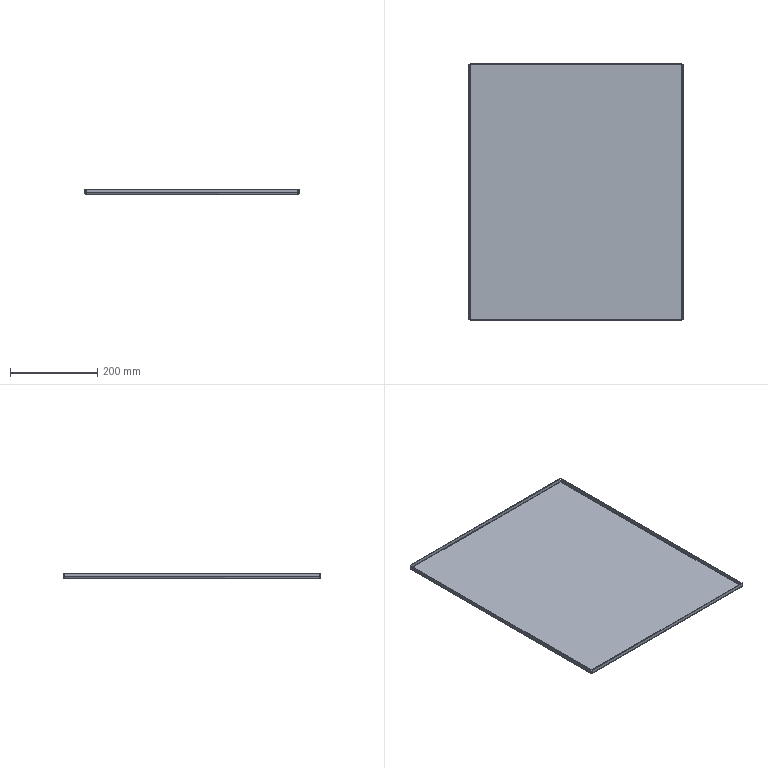Part | SolidWorks | features EdgeFlange 1, FlatPattern 1, SMBaseFlange 1, SheetMetal 1 | 1 solid | 38 faces | box 490 x 590 x 10 mm | volume 609167 mm3 | plane 22 | spline 8 | cylinder 8 | commonest cylinder face diameters 1.473 x4 5.473 x4
STEP:
#1=CARTESIAN_POINT('',(242.263,292.263,-2.));
#2=VERTEX_POINT('',#1);
#3=CARTESIAN_POINT('',(242.263,-292.263,-2.));
#4=VERTEX_POINT('',#3);
#5=CARTESIAN_POINT('',(242.263,292.293,-2.));
#6=DIRECTION('',(0.,-1.,0.));
#7=VECTOR('',#6,1000.);
#8=LINE('',#5,#7);
#9=EDGE_CURVE('',#2,#4,#8,.T.);
#10=ORIENTED_EDGE('',*,*,#9,.T.);
#11=CARTESIAN_POINT('',(-242.263,-292.263,-2.));
#12=VERTEX_POINT('',#11);
#13=CARTESIAN_POINT('',(242.293,-292.263,-2.));
#14=DIRECTION('',(-1.,0.,0.));
#15=VECTOR('',#14,1000.);
#16=LINE('',#13,#15);
#17=EDGE_CURVE('',#4,#12,#16,.T.);
#18=ORIENTED_EDGE('',*,*,#17,.T.);
#19=CARTESIAN_POINT('',(-242.263,292.263,-2.));
#20=VERTEX_POINT('',#19);
#21=CARTESIAN_POINT('',(-242.263,-292.293,-2.));
#22=DIRECTION('',(0.,1.,0.));
#23=VECTOR('',#22,1000.);
#24=LINE('',#21,#23);
#25=EDGE_CURVE('',#12,#20,#24,.T.);
#26=ORIENTED_EDGE('',*,*,#25,.T.);
#27=CARTESIAN_POINT('',(-242.293,292.263,-2.));
#28=DIRECTION('',(1.,0.,0.));
#29=VECTOR('',#28,1000.);
#30=LINE('',#27,#29);
#31=EDGE_CURVE('',#20,#2,#30,.T.);
#32=ORIENTED_EDGE('',*,*,#31,.T.);
#33=EDGE_LOOP('',(#10,#18,#26,#32));
#34=FACE_OUTER_BOUND('',#33,.T.);
#35=CARTESIAN_POINT('',(0.,0.,-2.));
#36=DIRECTION('',(0.,0.,-1.));
#37=DIRECTION('',(-1.,0.,0.));
#38=AXIS2_PLACEMENT_3D('',#35,#36,#37);
#39=PLANE('',#38);
#40=ADVANCED_FACE('',(#34),#39,.T.);
#41=CARTESIAN_POINT('',(242.263,-292.263,0.));
#42=VERTEX_POINT('',#41);
#43=CARTESIAN_POINT('',(-242.263,-292.263,0.));
#44=VERTEX_POINT('',#43);
#45=CARTESIAN_POINT('',(242.293,-292.263,0.));
#46=DIRECTION('',(-1.,0.,0.));
#47=VECTOR('',#46,1000.);
#48=LINE('',#45,#47);
#49=EDGE_CURVE('',#42,#44,#48,.T.);
#50=ORIENTED_EDGE('',*,*,#49,.F.);
#51=CARTESIAN_POINT('',(242.263,292.263,0.));
#52=VERTEX_POINT('',#51);
#53=CARTESIAN_POINT('',(242.263,292.293,0.));
#54=DIRECTION('',(0.,-1.,0.));
#55=VECTOR('',#54,1000.);
#56=LINE('',#53,#55);
#57=EDGE_CURVE('',#52,#42,#56,.T.);
#58=ORIENTED_EDGE('',*,*,#57,.F.);
#59=CARTESIAN_POINT('',(-242.263,292.263,0.));
#60=VERTEX_POINT('',#59);
#61=CARTESIAN_POINT('',(-242.293,292.263,0.));
#62=DIRECTION('',(1.,0.,0.));
#63=VECTOR('',#62,1000.);
#64=LINE('',#61,#63);
#65=EDGE_CURVE('',#60,#52,#64,.T.);
#66=ORIENTED_EDGE('',*,*,#65,.F.);
#67=CARTESIAN_POINT('',(-242.263,-292.293,0.));
#68=DIRECTION('',(0.,1.,0.));
#69=VECTOR('',#68,1000.);
#70=LINE('',#67,#69);
#71=EDGE_CURVE('',#44,#60,#70,.T.);
#72=ORIENTED_EDGE('',*,*,#71,.F.);
#73=EDGE_LOOP('',(#50,#58,#66,#72));
#74=FACE_OUTER_BOUND('',#73,.T.);
#75=CARTESIAN_POINT('',(0.,0.,0.));
#76=DIRECTION('',(0.,0.,-1.));
#77=DIRECTION('',(-1.,0.,0.));
#78=AXIS2_PLACEMENT_3D('',#75,#76,#77);
#79=PLANE('',#78);
#80=ADVANCED_FACE('',(#74),#79,.F.);
#81=CARTESIAN_POINT('',(242.293,295.,0.7366));
#82=VERTEX_POINT('',#81);
#83=CARTESIAN_POINT('',(242.293,293.,0.7366));
#84=VERTEX_POINT('',#83);
#85=CARTESIAN_POINT('',(242.293,293.,0.7366));
#86=DIRECTION('',(0.,-1.,0.));
#87=VECTOR('',#86,1000.);
#88=LINE('',#85,#87);
#89=EDGE_CURVE('',#82,#84,#88,.T.);
#90=ORIENTED_EDGE('',*,*,#89,.T.);
#91=CARTESIAN_POINT('',(242.263,292.263,0.));
#92=CARTESIAN_POINT('',(242.268,292.456,0.));
#93=CARTESIAN_POINT('',(242.273,292.648,0.07939));
#94=CARTESIAN_POINT('',(242.283,292.921,0.3521));
#95=CARTESIAN_POINT('',(242.288,293.,0.5438));
#96=CARTESIAN_POINT('',(242.293,293.,0.7366));
#97=B_SPLINE_CURVE_WITH_KNOTS('',3,(#91,#92,#93,#94,#95,#96),.UNSPECIFIED.,.F.,.F.,(4,2,4),(0.,0.5,1.),.UNSPECIFIED.);
#98=EDGE_CURVE('',#52,#84,#97,.T.);
#99=ORIENTED_EDGE('',*,*,#98,.F.);
#100=CARTESIAN_POINT('',(242.263,292.263,0.));
#101=DIRECTION('',(0.,0.,-1.));
#102=VECTOR('',#101,1000.);
#103=LINE('',#100,#102);
#104=EDGE_CURVE('',#52,#2,#103,.T.);
#105=ORIENTED_EDGE('',*,*,#104,.T.);
#106=CARTESIAN_POINT('',(242.263,292.263,-2.));
#107=CARTESIAN_POINT('',(242.266,292.622,-2.));
#108=CARTESIAN_POINT('',(242.268,292.98,-1.929));
#109=CARTESIAN_POINT('',(242.273,293.642,-1.655));
#110=CARTESIAN_POINT('',(242.276,293.945,-1.452));
#111=CARTESIAN_POINT('',(242.281,294.452,-0.9452));
#112=CARTESIAN_POINT('',(242.283,294.655,-0.6416));
#113=CARTESIAN_POINT('',(242.288,294.929,0.0203));
#114=CARTESIAN_POINT('',(242.29,295.,0.3784));
#115=CARTESIAN_POINT('',(242.293,295.,0.7366));
#116=B_SPLINE_CURVE_WITH_KNOTS('',3,(#106,#107,#108,#109,#110,#111,#112,#113,#114,#115),.UNSPECIFIED.,.F.,.F.,(4,2,2,2,4),(0.,0.25,0.5,0.75,1.),.UNSPECIFIED.);
#117=EDGE_CURVE('',#2,#82,#116,.T.);
#118=ORIENTED_EDGE('',*,*,#117,.T.);
#119=EDGE_LOOP('',(#90,#99,#105,#118));
#120=FACE_OUTER_BOUND('',#119,.T.);
#121=CARTESIAN_POINT('',(242.263,292.263,-2.02));
#122=CARTESIAN_POINT('',(242.266,292.624,-2.02));
#123=CARTESIAN_POINT('',(242.268,292.985,-1.948));
#124=CARTESIAN_POINT('',(242.273,293.652,-1.672));
#125=CARTESIAN_POINT('',(242.276,293.957,-1.468));
#126=CARTESIAN_POINT('',(242.281,294.468,-0.9575));
#127=CARTESIAN_POINT('',(242.283,294.672,-0.6517));
#128=CARTESIAN_POINT('',(242.288,294.948,0.01507));
#129=CARTESIAN_POINT('',(242.29,295.02,0.3757));
#130=CARTESIAN_POINT('',(242.293,295.02,0.7366));
#131=CARTESIAN_POINT('',(242.263,292.263,-2.));
#132=CARTESIAN_POINT('',(242.266,292.622,-2.));
#133=CARTESIAN_POINT('',(242.268,292.98,-1.929));
#134=CARTESIAN_POINT('',(242.273,293.642,-1.655));
#135=CARTESIAN_POINT('',(242.276,293.945,-1.452));
#136=CARTESIAN_POINT('',(242.281,294.452,-0.9452));
#137=CARTESIAN_POINT('',(242.283,294.655,-0.6416));
#138=CARTESIAN_POINT('',(242.288,294.929,0.0203));
#139=CARTESIAN_POINT('',(242.29,295.,0.3783));
#140=CARTESIAN_POINT('',(242.293,295.,0.7366));
#141=CARTESIAN_POINT('',(242.263,292.263,0.));
#142=CARTESIAN_POINT('',(242.266,292.36,0.));
#143=CARTESIAN_POINT('',(242.268,292.456,0.01917));
#144=CARTESIAN_POINT('',(242.273,292.634,0.09297));
#145=CARTESIAN_POINT('',(242.276,292.716,0.1476));
#146=CARTESIAN_POINT('',(242.281,292.852,0.2839));
#147=CARTESIAN_POINT('',(242.283,292.907,0.3656));
#148=CARTESIAN_POINT('',(242.288,292.981,0.5438));
#149=CARTESIAN_POINT('',(242.29,293.,0.6402));
#150=CARTESIAN_POINT('',(242.293,293.,0.7366));
#151=CARTESIAN_POINT('',(242.263,292.263,0.0202));
#152=CARTESIAN_POINT('',(242.266,292.357,0.0202));
#153=CARTESIAN_POINT('',(242.268,292.451,0.03885));
#154=CARTESIAN_POINT('',(242.273,292.624,0.1106));
#155=CARTESIAN_POINT('',(242.276,292.704,0.1637));
#156=CARTESIAN_POINT('',(242.281,292.836,0.2963));
#157=CARTESIAN_POINT('',(242.283,292.889,0.3758));
#158=CARTESIAN_POINT('',(242.288,292.961,0.5491));
#159=CARTESIAN_POINT('',(242.29,292.98,0.6428));
#160=CARTESIAN_POINT('',(242.293,292.98,0.7366));
#161=B_SPLINE_SURFACE_WITH_KNOTS('',1,3,((#121,#122,#123,#124,#125,#126,#127,#128,#129,#130),(#131,#132,#133,#134,#135,#136,#137,#138,#139,#140),(#141,#142,#143,#144,#145,#146,#147,#148,#149,#150),(#151,#152,#153,#154,#155,#156,#157,#158,#159,#160)),.UNSPECIFIED.,.F.,.F.,.F.,(2,1,1,2),(4,2,2,2,4),(-0.01,0.,1.,1.01),(0.,0.25,0.5,0.75,1.),.UNSPECIFIED.);
#162=ADVANCED_FACE('',(#120),#161,.F.);
#163=CARTESIAN_POINT('',(-242.293,293.,0.7366));
#164=VERTEX_POINT('',#163);
#165=CARTESIAN_POINT('',(-242.293,293.,0.7366));
#166=CARTESIAN_POINT('',(-242.288,293.,0.5438));
#167=CARTESIAN_POINT('',(-242.283,292.921,0.3521));
#168=CARTESIAN_POINT('',(-242.273,292.648,0.07939));
#169=CARTESIAN_POINT('',(-242.268,292.456,0.));
#170=CARTESIAN_POINT('',(-242.263,292.263,0.));
#171=B_SPLINE_CURVE_WITH_KNOTS('',3,(#165,#166,#167,#168,#169,#170),.UNSPECIFIED.,.F.,.F.,(4,2,4),(0.,0.5,1.),.UNSPECIFIED.);
#172=EDGE_CURVE('',#164,#60,#171,.T.);
#173=ORIENTED_EDGE('',*,*,#172,.F.);
#174=CARTESIAN_POINT('',(-242.293,295.,0.7366));
#175=VERTEX_POINT('',#174);
#176=CARTESIAN_POINT('',(-242.293,293.,0.7366));
#177=DIRECTION('',(0.,-1.,0.));
#178=VECTOR('',#177,1000.);
#179=LINE('',#176,#178);
#180=EDGE_CURVE('',#175,#164,#179,.T.);
#181=ORIENTED_EDGE('',*,*,#180,.F.);
#182=CARTESIAN_POINT('',(-242.293,295.,0.7366));
#183=CARTESIAN_POINT('',(-242.29,295.,0.3784));
#184=CARTESIAN_POINT('',(-242.288,294.929,0.0203));
#185=CARTESIAN_POINT('',(-242.283,294.655,-0.6416));
#186=CARTESIAN_POINT('',(-242.281,294.452,-0.9452));
#187=CARTESIAN_POINT('',(-242.276,293.945,-1.452));
#188=CARTESIAN_POINT('',(-242.273,293.642,-1.655));
#189=CARTESIAN_POINT('',(-242.268,292.98,-1.929));
#190=CARTESIAN_POINT('',(-242.266,292.622,-2.));
#191=CARTESIAN_POINT('',(-242.263,292.263,-2.));
#192=B_SPLINE_CURVE_WITH_KNOTS('',3,(#182,#183,#184,#185,#186,#187,#188,#189,#190,#191),.UNSPECIFIED.,.F.,.F.,(4,2,2,2,4),(0.,0.25,0.5,0.75,1.),.UNSPECIFIED.);
#193=EDGE_CURVE('',#175,#20,#192,.T.);
#194=ORIENTED_EDGE('',*,*,#193,.T.);
#195=CARTESIAN_POINT('',(-242.263,292.263,0.));
#196=DIRECTION('',(0.,0.,-1.));
#197=VECTOR('',#196,1000.);
#198=LINE('',#195,#197);
#199=EDGE_CURVE('',#60,#20,#198,.T.);
#200=ORIENTED_EDGE('',*,*,#199,.F.);
#201=EDGE_LOOP('',(#173,#181,#194,#200));
#202=FACE_OUTER_BOUND('',#201,.T.);
#203=CARTESIAN_POINT('',(-242.293,295.02,0.7366));
#204=CARTESIAN_POINT('',(-242.29,295.02,0.3757));
#205=CARTESIAN_POINT('',(-242.288,294.948,0.01507));
#206=CARTESIAN_POINT('',(-242.283,294.672,-0.6517));
#207=CARTESIAN_POINT('',(-242.281,294.468,-0.9575));
#208=CARTESIAN_POINT('',(-242.276,293.957,-1.468));
#209=CARTESIAN_POINT('',(-242.273,293.652,-1.672));
#210=CARTESIAN_POINT('',(-242.268,292.985,-1.948));
#211=CARTESIAN_POINT('',(-242.266,292.624,-2.02));
#212=CARTESIAN_POINT('',(-242.263,292.263,-2.02));
#213=CARTESIAN_POINT('',(-242.293,295.,0.7366));
#214=CARTESIAN_POINT('',(-242.29,295.,0.3783));
#215=CARTESIAN_POINT('',(-242.288,294.929,0.0203));
#216=CARTESIAN_POINT('',(-242.283,294.655,-0.6416));
#217=CARTESIAN_POINT('',(-242.281,294.452,-0.9452));
#218=CARTESIAN_POINT('',(-242.276,293.945,-1.452));
#219=CARTESIAN_POINT('',(-242.273,293.642,-1.655));
#220=CARTESIAN_POINT('',(-242.268,292.98,-1.929));
#221=CARTESIAN_POINT('',(-242.266,292.622,-2.));
#222=CARTESIAN_POINT('',(-242.263,292.263,-2.));
#223=CARTESIAN_POINT('',(-242.293,293.,0.7366));
#224=CARTESIAN_POINT('',(-242.29,293.,0.6402));
#225=CARTESIAN_POINT('',(-242.288,292.981,0.5438));
#226=CARTESIAN_POINT('',(-242.283,292.907,0.3656));
#227=CARTESIAN_POINT('',(-242.281,292.852,0.2839));
#228=CARTESIAN_POINT('',(-242.276,292.716,0.1476));
#229=CARTESIAN_POINT('',(-242.273,292.634,0.09297));
#230=CARTESIAN_POINT('',(-242.268,292.456,0.01917));
#231=CARTESIAN_POINT('',(-242.266,292.36,0.));
#232=CARTESIAN_POINT('',(-242.263,292.263,0.));
#233=CARTESIAN_POINT('',(-242.293,292.98,0.7366));
#234=CARTESIAN_POINT('',(-242.29,292.98,0.6428));
#235=CARTESIAN_POINT('',(-242.288,292.961,0.5491));
#236=CARTESIAN_POINT('',(-242.283,292.889,0.3758));
#237=CARTESIAN_POINT('',(-242.281,292.836,0.2963));
#238=CARTESIAN_POINT('',(-242.276,292.704,0.1637));
#239=CARTESIAN_POINT('',(-242.273,292.624,0.1106));
#240=CARTESIAN_POINT('',(-242.268,292.451,0.03885));
#241=CARTESIAN_POINT('',(-242.266,292.357,0.0202));
#242=CARTESIAN_POINT('',(-242.263,292.263,0.0202));
#243=B_SPLINE_SURFACE_WITH_KNOTS('',1,3,((#203,#204,#205,#206,#207,#208,#209,#210,#211,#212),(#213,#214,#215,#216,#217,#218,#219,#220,#221,#222),(#223,#224,#225,#226,#227,#228,#229,#230,#231,#232),(#233,#234,#235,#236,#237,#238,#239,#240,#241,#242)),.UNSPECIFIED.,.F.,.F.,.F.,(2,1,1,2),(4,2,2,2,4),(-0.01,0.,1.,1.01),(0.,0.25,0.5,0.75,1.),.UNSPECIFIED.);
#244=ADVANCED_FACE('',(#202),#243,.F.);
#245=ORIENTED_EDGE('',*,*,#31,.F.);
#246=ORIENTED_EDGE('',*,*,#193,.F.);
#247=CARTESIAN_POINT('',(245.,295.,0.7366));
#248=DIRECTION('',(1.,0.,0.));
#249=VECTOR('',#248,1000.);
#250=LINE('',#247,#249);
#251=EDGE_CURVE('',#175,#82,#250,.T.);
#252=ORIENTED_EDGE('',*,*,#251,.T.);
#253=ORIENTED_EDGE('',*,*,#117,.F.);
#254=EDGE_LOOP('',(#245,#246,#252,#253));
#255=FACE_OUTER_BOUND('',#254,.T.);
#256=CARTESIAN_POINT('',(-242.293,292.263,0.7366));
#257=DIRECTION('',(-1.,0.,0.));
#258=DIRECTION('',(0.,1.,0.));
#259=AXIS2_PLACEMENT_3D('',#256,#257,#258);
#260=CYLINDRICAL_SURFACE('',#259,2.737);
#261=ADVANCED_FACE('',(#255),#260,.T.);
#262=ORIENTED_EDGE('',*,*,#65,.T.);
#263=ORIENTED_EDGE('',*,*,#98,.T.);
#264=CARTESIAN_POINT('',(245.,293.,0.7366));
#265=DIRECTION('',(-1.,0.,0.));
#266=VECTOR('',#265,1000.);
#267=LINE('',#264,#266);
#268=EDGE_CURVE('',#84,#164,#267,.T.);
#269=ORIENTED_EDGE('',*,*,#268,.T.);
#270=ORIENTED_EDGE('',*,*,#172,.T.);
#271=EDGE_LOOP('',(#262,#263,#269,#270));
#272=FACE_OUTER_BOUND('',#271,.T.);
#273=CARTESIAN_POINT('',(-242.293,292.263,0.7366));
#274=DIRECTION('',(-1.,0.,0.));
#275=DIRECTION('',(0.,1.,0.));
#276=AXIS2_PLACEMENT_3D('',#273,#274,#275);
#277=CYLINDRICAL_SURFACE('',#276,0.7366);
#278=ADVANCED_FACE('',(#272),#277,.F.);
#279=CARTESIAN_POINT('',(242.293,295.,8.));
#280=VERTEX_POINT('',#279);
#281=CARTESIAN_POINT('',(242.293,295.,0.));
#282=DIRECTION('',(0.,0.,1.));
#283=VECTOR('',#282,1000.);
#284=LINE('',#281,#283);
#285=EDGE_CURVE('',#82,#280,#284,.T.);
#286=ORIENTED_EDGE('',*,*,#285,.T.);
#287=CARTESIAN_POINT('',(242.293,293.,8.));
#288=VERTEX_POINT('',#287);
#289=CARTESIAN_POINT('',(242.293,293.,8.));
#290=DIRECTION('',(0.,-1.,0.));
#291=VECTOR('',#290,1000.);
#292=LINE('',#289,#291);
#293=EDGE_CURVE('',#280,#288,#292,.T.);
#294=ORIENTED_EDGE('',*,*,#293,.T.);
#295=CARTESIAN_POINT('',(242.293,293.,0.));
#296=DIRECTION('',(0.,0.,1.));
#297=VECTOR('',#296,1000.);
#298=LINE('',#295,#297);
#299=EDGE_CURVE('',#84,#288,#298,.T.);
#300=ORIENTED_EDGE('',*,*,#299,.F.);
#301=ORIENTED_EDGE('',*,*,#89,.F.);
#302=EDGE_LOOP('',(#286,#294,#300,#301));
#303=FACE_OUTER_BOUND('',#302,.T.);
#304=CARTESIAN_POINT('',(242.293,293.,0.));
#305=DIRECTION('',(1.,0.,0.));
#306=DIRECTION('',(0.,0.,-1.));
#307=AXIS2_PLACEMENT_3D('',#304,#305,#306);
#308=PLANE('',#307);
#309=ADVANCED_FACE('',(#303),#308,.T.);
#310=ORIENTED_EDGE('',*,*,#251,.F.);
#311=CARTESIAN_POINT('',(-242.293,295.,8.));
#312=VERTEX_POINT('',#311);
#313=CARTESIAN_POINT('',(-242.293,295.,0.));
#314=DIRECTION('',(0.,0.,1.));
#315=VECTOR('',#314,1000.);
#316=LINE('',#313,#315);
#317=EDGE_CURVE('',#175,#312,#316,.T.);
#318=ORIENTED_EDGE('',*,*,#317,.T.);
#319=CARTESIAN_POINT('',(0.,295.,8.));
#320=DIRECTION('',(1.,0.,0.));
#321=VECTOR('',#320,1000.);
#322=LINE('',#319,#321);
#323=EDGE_CURVE('',#312,#280,#322,.T.);
#324=ORIENTED_EDGE('',*,*,#323,.T.);
#325=ORIENTED_EDGE('',*,*,#285,.F.);
#326=EDGE_LOOP('',(#310,#318,#324,#325));
#327=FACE_OUTER_BOUND('',#326,.T.);
#328=CARTESIAN_POINT('',(0.,295.,0.));
#329=DIRECTION('',(0.,-1.,0.));
#330=DIRECTION('',(0.,0.,-1.));
#331=AXIS2_PLACEMENT_3D('',#328,#329,#330);
#332=PLANE('',#331);
#333=ADVANCED_FACE('',(#327),#332,.F.);
#334=CARTESIAN_POINT('',(-242.293,293.,8.));
#335=VERTEX_POINT('',#334);
#336=CARTESIAN_POINT('',(-242.293,293.,0.));
#337=DIRECTION('',(0.,0.,1.));
#338=VECTOR('',#337,1000.);
#339=LINE('',#336,#338);
#340=EDGE_CURVE('',#164,#335,#339,.T.);
#341=ORIENTED_EDGE('',*,*,#340,.F.);
#342=ORIENTED_EDGE('',*,*,#268,.F.);
#343=ORIENTED_EDGE('',*,*,#299,.T.);
#344=CARTESIAN_POINT('',(245.,293.,8.));
#345=DIRECTION('',(1.,0.,0.));
#346=VECTOR('',#345,1000.);
#347=LINE('',#344,#346);
#348=EDGE_CURVE('',#335,#288,#347,.T.);
#349=ORIENTED_EDGE('',*,*,#348,.F.);
#350=EDGE_LOOP('',(#341,#342,#343,#349));
#351=FACE_OUTER_BOUND('',#350,.T.);
#352=CARTESIAN_POINT('',(0.,293.,0.));
#353=DIRECTION('',(0.,-1.,0.));
#354=DIRECTION('',(0.,0.,-1.));
#355=AXIS2_PLACEMENT_3D('',#352,#353,#354);
#356=PLANE('',#355);
#357=ADVANCED_FACE('',(#351),#356,.T.);
#358=ORIENTED_EDGE('',*,*,#323,.F.);
#359=CARTESIAN_POINT('',(-242.293,295.,8.));
#360=DIRECTION('',(0.,-1.,0.));
#361=VECTOR('',#360,1000.);
#362=LINE('',#359,#361);
#363=EDGE_CURVE('',#312,#335,#362,.T.);
#364=ORIENTED_EDGE('',*,*,#363,.T.);
#365=ORIENTED_EDGE('',*,*,#348,.T.);
#366=ORIENTED_EDGE('',*,*,#293,.F.);
#367=EDGE_LOOP('',(#358,#364,#365,#366));
#368=FACE_OUTER_BOUND('',#367,.T.);
#369=CARTESIAN_POINT('',(245.,295.,8.));
#370=DIRECTION('',(0.,0.,-1.));
#371=DIRECTION('',(0.,1.,0.));
#372=AXIS2_PLACEMENT_3D('',#369,#370,#371);
#373=PLANE('',#372);
#374=ADVANCED_FACE('',(#368),#373,.F.);
#375=ORIENTED_EDGE('',*,*,#363,.F.);
#376=ORIENTED_EDGE('',*,*,#317,.F.);
#377=ORIENTED_EDGE('',*,*,#180,.T.);
#378=ORIENTED_EDGE('',*,*,#340,.T.);
#379=EDGE_LOOP('',(#375,#376,#377,#378));
#380=FACE_OUTER_BOUND('',#379,.T.);
#381=CARTESIAN_POINT('',(-242.293,293.,0.));
#382=DIRECTION('',(1.,0.,0.));
#383=DIRECTION('',(0.,0.,-1.));
#384=AXIS2_PLACEMENT_3D('',#381,#382,#383);
#385=PLANE('',#384);
#386=ADVANCED_FACE('',(#380),#385,.F.);
#387=CARTESIAN_POINT('',(245.,-292.293,0.7366));
#388=VERTEX_POINT('',#387);
#389=CARTESIAN_POINT('',(243.,-292.293,0.7366));
#390=VERTEX_POINT('',#389);
#391=CARTESIAN_POINT('',(243.,-292.293,0.7366));
#392=DIRECTION('',(-1.,0.,0.));
#393=VECTOR('',#392,1000.);
#394=LINE('',#391,#393);
#395=EDGE_CURVE('',#388,#390,#394,.T.);
#396=ORIENTED_EDGE('',*,*,#395,.T.);
#397=CARTESIAN_POINT('',(242.263,-292.263,0.));
#398=CARTESIAN_POINT('',(242.456,-292.268,0.));
#399=CARTESIAN_POINT('',(242.648,-292.273,0.07939));
#400=CARTESIAN_POINT('',(242.921,-292.283,0.3521));
#401=CARTESIAN_POINT('',(243.,-292.288,0.5438));
#402=CARTESIAN_POINT('',(243.,-292.293,0.7366));
#403=B_SPLINE_CURVE_WITH_KNOTS('',3,(#397,#398,#399,#400,#401,#402),.UNSPECIFIED.,.F.,.F.,(4,2,4),(0.,0.5,1.),.UNSPECIFIED.);
#404=EDGE_CURVE('',#42,#390,#403,.T.);
#405=ORIENTED_EDGE('',*,*,#404,.F.);
#406=CARTESIAN_POINT('',(242.263,-292.263,0.));
#407=DIRECTION('',(0.,0.,-1.));
#408=VECTOR('',#407,1000.);
#409=LINE('',#406,#408);
#410=EDGE_CURVE('',#42,#4,#409,.T.);
#411=ORIENTED_EDGE('',*,*,#410,.T.);
#412=CARTESIAN_POINT('',(242.263,-292.263,-2.));
#413=CARTESIAN_POINT('',(242.622,-292.266,-2.));
#414=CARTESIAN_POINT('',(242.98,-292.268,-1.929));
#415=CARTESIAN_POINT('',(243.642,-292.273,-1.655));
#416=CARTESIAN_POINT('',(243.945,-292.276,-1.452));
#417=CARTESIAN_POINT('',(244.452,-292.281,-0.9452));
#418=CARTESIAN_POINT('',(244.655,-292.283,-0.6416));
#419=CARTESIAN_POINT('',(244.929,-292.288,0.0203));
#420=CARTESIAN_POINT('',(245.,-292.29,0.3784));
#421=CARTESIAN_POINT('',(245.,-292.293,0.7366));
#422=B_SPLINE_CURVE_WITH_KNOTS('',3,(#412,#413,#414,#415,#416,#417,#418,#419,#420,#421),.UNSPECIFIED.,.F.,.F.,(4,2,2,2,4),(0.,0.25,0.5,0.75,1.),.UNSPECIFIED.);
#423=EDGE_CURVE('',#4,#388,#422,.T.);
#424=ORIENTED_EDGE('',*,*,#423,.T.);
#425=EDGE_LOOP('',(#396,#405,#411,#424));
#426=FACE_OUTER_BOUND('',#425,.T.);
#427=CARTESIAN_POINT('',(242.263,-292.263,-2.02));
#428=CARTESIAN_POINT('',(242.624,-292.266,-2.02));
#429=CARTESIAN_POINT('',(242.985,-292.268,-1.948));
#430=CARTESIAN_POINT('',(243.652,-292.273,-1.672));
#431=CARTESIAN_POINT('',(243.957,-292.276,-1.468));
#432=CARTESIAN_POINT('',(244.468,-292.281,-0.9575));
#433=CARTESIAN_POINT('',(244.672,-292.283,-0.6517));
#434=CARTESIAN_POINT('',(244.948,-292.288,0.01507));
#435=CARTESIAN_POINT('',(245.02,-292.29,0.3757));
#436=CARTESIAN_POINT('',(245.02,-292.293,0.7366));
#437=CARTESIAN_POINT('',(242.263,-292.263,-2.));
#438=CARTESIAN_POINT('',(242.622,-292.266,-2.));
#439=CARTESIAN_POINT('',(242.98,-292.268,-1.929));
#440=CARTESIAN_POINT('',(243.642,-292.273,-1.655));
#441=CARTESIAN_POINT('',(243.945,-292.276,-1.452));
#442=CARTESIAN_POINT('',(244.452,-292.281,-0.9452));
#443=CARTESIAN_POINT('',(244.655,-292.283,-0.6416));
#444=CARTESIAN_POINT('',(244.929,-292.288,0.0203));
#445=CARTESIAN_POINT('',(245.,-292.29,0.3783));
#446=CARTESIAN_POINT('',(245.,-292.293,0.7366));
#447=CARTESIAN_POINT('',(242.263,-292.263,0.));
#448=CARTESIAN_POINT('',(242.36,-292.266,0.));
#449=CARTESIAN_POINT('',(242.456,-292.268,0.01917));
#450=CARTESIAN_POINT('',(242.634,-292.273,0.09297));
#451=CARTESIAN_POINT('',(242.716,-292.276,0.1476));
#452=CARTESIAN_POINT('',(242.852,-292.281,0.2839));
#453=CARTESIAN_POINT('',(242.907,-292.283,0.3656));
#454=CARTESIAN_POINT('',(242.981,-292.288,0.5438));
#455=CARTESIAN_POINT('',(243.,-292.29,0.6402));
#456=CARTESIAN_POINT('',(243.,-292.293,0.7366));
#457=CARTESIAN_POINT('',(242.263,-292.263,0.0202));
#458=CARTESIAN_POINT('',(242.357,-292.266,0.0202));
#459=CARTESIAN_POINT('',(242.451,-292.268,0.03885));
#460=CARTESIAN_POINT('',(242.624,-292.273,0.1106));
#461=CARTESIAN_POINT('',(242.704,-292.276,0.1637));
#462=CARTESIAN_POINT('',(242.836,-292.281,0.2963));
#463=CARTESIAN_POINT('',(242.889,-292.283,0.3758));
#464=CARTESIAN_POINT('',(242.961,-292.288,0.5491));
#465=CARTESIAN_POINT('',(242.98,-292.29,0.6428));
#466=CARTESIAN_POINT('',(242.98,-292.293,0.7366));
#467=B_SPLINE_SURFACE_WITH_KNOTS('',1,3,((#427,#428,#429,#430,#431,#432,#433,#434,#435,#436),(#437,#438,#439,#440,#441,#442,#443,#444,#445,#446),(#447,#448,#449,#450,#451,#452,#453,#454,#455,#456),(#457,#458,#459,#460,#461,#462,#463,#464,#465,#466)),.UNSPECIFIED.,.F.,.F.,.F.,(2,1,1,2),(4,2,2,2,4),(-0.01,0.,1.,1.01),(0.,0.25,0.5,0.75,1.),.UNSPECIFIED.);
#468=ADVANCED_FACE('',(#426),#467,.F.);
#469=CARTESIAN_POINT('',(243.,292.293,0.7366));
#470=VERTEX_POINT('',#469);
#471=CARTESIAN_POINT('',(243.,292.293,0.7366));
#472=CARTESIAN_POINT('',(243.,292.288,0.5438));
#473=CARTESIAN_POINT('',(242.921,292.283,0.3521));
#474=CARTESIAN_POINT('',(242.648,292.273,0.07939));
#475=CARTESIAN_POINT('',(242.456,292.268,0.));
#476=CARTESIAN_POINT('',(242.263,292.263,0.));
#477=B_SPLINE_CURVE_WITH_KNOTS('',3,(#471,#472,#473,#474,#475,#476),.UNSPECIFIED.,.F.,.F.,(4,2,4),(0.,0.5,1.),.UNSPECIFIED.);
#478=EDGE_CURVE('',#470,#52,#477,.T.);
#479=ORIENTED_EDGE('',*,*,#478,.F.);
#480=CARTESIAN_POINT('',(245.,292.293,0.7366));
#481=VERTEX_POINT('',#480);
#482=CARTESIAN_POINT('',(243.,292.293,0.7366));
#483=DIRECTION('',(-1.,0.,0.));
#484=VECTOR('',#483,1000.);
#485=LINE('',#482,#484);
#486=EDGE_CURVE('',#481,#470,#485,.T.);
#487=ORIENTED_EDGE('',*,*,#486,.F.);
#488=CARTESIAN_POINT('',(245.,292.293,0.7366));
#489=CARTESIAN_POINT('',(245.,292.29,0.3784));
#490=CARTESIAN_POINT('',(244.929,292.288,0.0203));
#491=CARTESIAN_POINT('',(244.655,292.283,-0.6416));
#492=CARTESIAN_POINT('',(244.452,292.281,-0.9452));
#493=CARTESIAN_POINT('',(243.945,292.276,-1.452));
#494=CARTESIAN_POINT('',(243.642,292.273,-1.655));
#495=CARTESIAN_POINT('',(242.98,292.268,-1.929));
#496=CARTESIAN_POINT('',(242.622,292.266,-2.));
#497=CARTESIAN_POINT('',(242.263,292.263,-2.));
#498=B_SPLINE_CURVE_WITH_KNOTS('',3,(#488,#489,#490,#491,#492,#493,#494,#495,#496,#497),.UNSPECIFIED.,.F.,.F.,(4,2,2,2,4),(0.,0.25,0.5,0.75,1.),.UNSPECIFIED.);
#499=EDGE_CURVE('',#481,#2,#498,.T.);
#500=ORIENTED_EDGE('',*,*,#499,.T.);
#501=ORIENTED_EDGE('',*,*,#104,.F.);
#502=EDGE_LOOP('',(#479,#487,#500,#501));
#503=FACE_OUTER_BOUND('',#502,.T.);
#504=CARTESIAN_POINT('',(245.02,292.293,0.7366));
#505=CARTESIAN_POINT('',(245.02,292.29,0.3757));
#506=CARTESIAN_POINT('',(244.948,292.288,0.01507));
#507=CARTESIAN_POINT('',(244.672,292.283,-0.6517));
#508=CARTESIAN_POINT('',(244.468,292.281,-0.9575));
#509=CARTESIAN_POINT('',(243.957,292.276,-1.468));
#510=CARTESIAN_POINT('',(243.652,292.273,-1.672));
#511=CARTESIAN_POINT('',(242.985,292.268,-1.948));
#512=CARTESIAN_POINT('',(242.624,292.266,-2.02));
#513=CARTESIAN_POINT('',(242.263,292.263,-2.02));
#514=CARTESIAN_POINT('',(245.,292.293,0.7366));
#515=CARTESIAN_POINT('',(245.,292.29,0.3783));
#516=CARTESIAN_POINT('',(244.929,292.288,0.0203));
#517=CARTESIAN_POINT('',(244.655,292.283,-0.6416));
#518=CARTESIAN_POINT('',(244.452,292.281,-0.9452));
#519=CARTESIAN_POINT('',(243.945,292.276,-1.452));
#520=CARTESIAN_POINT('',(243.642,292.273,-1.655));
#521=CARTESIAN_POINT('',(242.98,292.268,-1.929));
#522=CARTESIAN_POINT('',(242.622,292.266,-2.));
#523=CARTESIAN_POINT('',(242.263,292.263,-2.));
#524=CARTESIAN_POINT('',(243.,292.293,0.7366));
#525=CARTESIAN_POINT('',(243.,292.29,0.6402));
#526=CARTESIAN_POINT('',(242.981,292.288,0.5438));
#527=CARTESIAN_POINT('',(242.907,292.283,0.3656));
#528=CARTESIAN_POINT('',(242.852,292.281,0.2839));
#529=CARTESIAN_POINT('',(242.716,292.276,0.1476));
#530=CARTESIAN_POINT('',(242.634,292.273,0.09297));
#531=CARTESIAN_POINT('',(242.456,292.268,0.01917));
#532=CARTESIAN_POINT('',(242.36,292.266,0.));
#533=CARTESIAN_POINT('',(242.263,292.263,0.));
#534=CARTESIAN_POINT('',(242.98,292.293,0.7366));
#535=CARTESIAN_POINT('',(242.98,292.29,0.6428));
#536=CARTESIAN_POINT('',(242.961,292.288,0.5491));
#537=CARTESIAN_POINT('',(242.889,292.283,0.3758));
#538=CARTESIAN_POINT('',(242.836,292.281,0.2963));
#539=CARTESIAN_POINT('',(242.704,292.276,0.1637));
#540=CARTESIAN_POINT('',(242.624,292.273,0.1106));
#541=CARTESIAN_POINT('',(242.451,292.268,0.03885));
#542=CARTESIAN_POINT('',(242.357,292.266,0.0202));
#543=CARTESIAN_POINT('',(242.263,292.263,0.0202));
#544=B_SPLINE_SURFACE_WITH_KNOTS('',1,3,((#504,#505,#506,#507,#508,#509,#510,#511,#512,#513),(#514,#515,#516,#517,#518,#519,#520,#521,#522,#523),(#524,#525,#526,#527,#528,#529,#530,#531,#532,#533),(#534,#535,#536,#537,#538,#539,#540,#541,#542,#543)),.UNSPECIFIED.,.F.,.F.,.F.,(2,1,1,2),(4,2,2,2,4),(-0.01,0.,1.,1.01),(0.,0.25,0.5,0.75,1.),.UNSPECIFIED.);
#545=ADVANCED_FACE('',(#503),#544,.F.);
#546=ORIENTED_EDGE('',*,*,#9,.F.);
#547=ORIENTED_EDGE('',*,*,#499,.F.);
#548=CARTESIAN_POINT('',(245.,-295.,0.7366));
#549=DIRECTION('',(0.,-1.,0.));
#550=VECTOR('',#549,1000.);
#551=LINE('',#548,#550);
#552=EDGE_CURVE('',#481,#388,#551,.T.);
#553=ORIENTED_EDGE('',*,*,#552,.T.);
#554=ORIENTED_EDGE('',*,*,#423,.F.);
#555=EDGE_LOOP('',(#546,#547,#553,#554));
#556=FACE_OUTER_BOUND('',#555,.T.);
#557=CARTESIAN_POINT('',(242.263,292.293,0.7366));
#558=DIRECTION('',(0.,1.,0.));
#559=DIRECTION('',(1.,0.,0.));
#560=AXIS2_PLACEMENT_3D('',#557,#558,#559);
#561=CYLINDRICAL_SURFACE('',#560,2.737);
#562=ADVANCED_FACE('',(#556),#561,.T.);
#563=ORIENTED_EDGE('',*,*,#57,.T.);
#564=ORIENTED_EDGE('',*,*,#404,.T.);
#565=CARTESIAN_POINT('',(243.,-295.,0.7366));
#566=DIRECTION('',(0.,1.,0.));
#567=VECTOR('',#566,1000.);
#568=LINE('',#565,#567);
#569=EDGE_CURVE('',#390,#470,#568,.T.);
#570=ORIENTED_EDGE('',*,*,#569,.T.);
#571=ORIENTED_EDGE('',*,*,#478,.T.);
#572=EDGE_LOOP('',(#563,#564,#570,#571));
#573=FACE_OUTER_BOUND('',#572,.T.);
#574=CARTESIAN_POINT('',(242.263,292.293,0.7366));
#575=DIRECTION('',(0.,1.,0.));
#576=DIRECTION('',(1.,0.,0.));
#577=AXIS2_PLACEMENT_3D('',#574,#575,#576);
#578=CYLINDRICAL_SURFACE('',#577,0.7366);
#579=ADVANCED_FACE('',(#573),#578,.F.);
#580=CARTESIAN_POINT('',(245.,-292.293,8.));
#581=VERTEX_POINT('',#580);
#582=CARTESIAN_POINT('',(245.,-292.293,0.));
#583=DIRECTION('',(0.,0.,1.));
#584=VECTOR('',#583,1000.);
#585=LINE('',#582,#584);
#586=EDGE_CURVE('',#388,#581,#585,.T.);
#587=ORIENTED_EDGE('',*,*,#586,.T.);
#588=CARTESIAN_POINT('',(243.,-292.293,8.));
#589=VERTEX_POINT('',#588);
#590=CARTESIAN_POINT('',(243.,-292.293,8.));
#591=DIRECTION('',(-1.,0.,0.));
#592=VECTOR('',#591,1000.);
#593=LINE('',#590,#592);
#594=EDGE_CURVE('',#581,#589,#593,.T.);
#595=ORIENTED_EDGE('',*,*,#594,.T.);
#596=CARTESIAN_POINT('',(243.,-292.293,0.));
#597=DIRECTION('',(0.,0.,1.));
#598=VECTOR('',#597,1000.);
#599=LINE('',#596,#598);
#600=EDGE_CURVE('',#390,#589,#599,.T.);
#601=ORIENTED_EDGE('',*,*,#600,.F.);
#602=ORIENTED_EDGE('',*,*,#395,.F.);
#603=EDGE_LOOP('',(#587,#595,#601,#602));
#604=FACE_OUTER_BOUND('',#603,.T.);
#605=CARTESIAN_POINT('',(243.,-292.293,0.));
#606=DIRECTION('',(0.,-1.,0.));
#607=DIRECTION('',(0.,0.,-1.));
#608=AXIS2_PLACEMENT_3D('',#605,#606,#607);
#609=PLANE('',#608);
#610=ADVANCED_FACE('',(#604),#609,.T.);
#611=ORIENTED_EDGE('',*,*,#552,.F.);
#612=CARTESIAN_POINT('',(245.,292.293,8.));
#613=VERTEX_POINT('',#612);
#614=CARTESIAN_POINT('',(245.,292.293,0.));
#615=DIRECTION('',(0.,0.,1.));
#616=VECTOR('',#615,1000.);
#617=LINE('',#614,#616);
#618=EDGE_CURVE('',#481,#613,#617,.T.);
#619=ORIENTED_EDGE('',*,*,#618,.T.);
#620=CARTESIAN_POINT('',(245.,0.,8.));
#621=DIRECTION('',(0.,-1.,0.));
#622=VECTOR('',#621,1000.);
#623=LINE('',#620,#622);
#624=EDGE_CURVE('',#613,#581,#623,.T.);
#625=ORIENTED_EDGE('',*,*,#624,.T.);
#626=ORIENTED_EDGE('',*,*,#586,.F.);
#627=EDGE_LOOP('',(#611,#619,#625,#626));
#628=FACE_OUTER_BOUND('',#627,.T.);
#629=CARTESIAN_POINT('',(245.,0.,0.));
#630=DIRECTION('',(-1.,0.,0.));
#631=DIRECTION('',(0.,0.,1.));
#632=AXIS2_PLACEMENT_3D('',#629,#630,#631);
#633=PLANE('',#632);
#634=ADVANCED_FACE('',(#628),#633,.F.);
#635=CARTESIAN_POINT('',(243.,292.293,8.));
#636=VERTEX_POINT('',#635);
#637=CARTESIAN_POINT('',(243.,292.293,0.));
#638=DIRECTION('',(0.,0.,1.));
#639=VECTOR('',#638,1000.);
#640=LINE('',#637,#639);
#641=EDGE_CURVE('',#470,#636,#640,.T.);
#642=ORIENTED_EDGE('',*,*,#641,.F.);
#643=ORIENTED_EDGE('',*,*,#569,.F.);
#644=ORIENTED_EDGE('',*,*,#600,.T.);
#645=CARTESIAN_POINT('',(243.,-295.,8.));
#646=DIRECTION('',(0.,-1.,0.));
#647=VECTOR('',#646,1000.);
#648=LINE('',#645,#647);
#649=EDGE_CURVE('',#636,#589,#648,.T.);
#650=ORIENTED_EDGE('',*,*,#649,.F.);
#651=EDGE_LOOP('',(#642,#643,#644,#650));
#652=FACE_OUTER_BOUND('',#651,.T.);
#653=CARTESIAN_POINT('',(243.,0.,0.));
#654=DIRECTION('',(-1.,0.,0.));
#655=DIRECTION('',(0.,0.,1.));
#656=AXIS2_PLACEMENT_3D('',#653,#654,#655);
#657=PLANE('',#656);
#658=ADVANCED_FACE('',(#652),#657,.T.);
#659=ORIENTED_EDGE('',*,*,#624,.F.);
#660=CARTESIAN_POINT('',(245.,292.293,8.));
#661=DIRECTION('',(-1.,0.,0.));
#662=VECTOR('',#661,1000.);
#663=LINE('',#660,#662);
#664=EDGE_CURVE('',#613,#636,#663,.T.);
#665=ORIENTED_EDGE('',*,*,#664,.T.);
#666=ORIENTED_EDGE('',*,*,#649,.T.);
#667=ORIENTED_EDGE('',*,*,#594,.F.);
#668=EDGE_LOOP('',(#659,#665,#666,#667));
#669=FACE_OUTER_BOUND('',#668,.T.);
#670=CARTESIAN_POINT('',(245.,-295.,8.));
#671=DIRECTION('',(0.,0.,-1.));
#672=DIRECTION('',(-1.,0.,0.));
#673=AXIS2_PLACEMENT_3D('',#670,#671,#672);
#674=PLANE('',#673);
#675=ADVANCED_FACE('',(#669),#674,.F.);
#676=ORIENTED_EDGE('',*,*,#664,.F.);
#677=ORIENTED_EDGE('',*,*,#618,.F.);
#678=ORIENTED_EDGE('',*,*,#486,.T.);
#679=ORIENTED_EDGE('',*,*,#641,.T.);
#680=EDGE_LOOP('',(#676,#677,#678,#679));
#681=FACE_OUTER_BOUND('',#680,.T.);
#682=CARTESIAN_POINT('',(243.,292.293,0.));
#683=DIRECTION('',(0.,-1.,0.));
#684=DIRECTION('',(0.,0.,-1.));
#685=AXIS2_PLACEMENT_3D('',#682,#683,#684);
#686=PLANE('',#685);
#687=ADVANCED_FACE('',(#681),#686,.F.);
#688=CARTESIAN_POINT('',(-245.,292.293,0.7366));
#689=VERTEX_POINT('',#688);
#690=CARTESIAN_POINT('',(-243.,292.293,0.7366));
#691=VERTEX_POINT('',#690);
#692=CARTESIAN_POINT('',(-243.,292.293,0.7366));
#693=DIRECTION('',(1.,0.,0.));
#694=VECTOR('',#693,1000.);
#695=LINE('',#692,#694);
#696=EDGE_CURVE('',#689,#691,#695,.T.);
#697=ORIENTED_EDGE('',*,*,#696,.T.);
#698=CARTESIAN_POINT('',(-242.263,292.263,0.));
#699=CARTESIAN_POINT('',(-242.456,292.268,0.));
#700=CARTESIAN_POINT('',(-242.648,292.273,0.07939));
#701=CARTESIAN_POINT('',(-242.921,292.283,0.3521));
#702=CARTESIAN_POINT('',(-243.,292.288,0.5438));
#703=CARTESIAN_POINT('',(-243.,292.293,0.7366));
#704=B_SPLINE_CURVE_WITH_KNOTS('',3,(#698,#699,#700,#701,#702,#703),.UNSPECIFIED.,.F.,.F.,(4,2,4),(0.,0.5,1.),.UNSPECIFIED.);
#705=EDGE_CURVE('',#60,#691,#704,.T.);
#706=ORIENTED_EDGE('',*,*,#705,.F.);
#707=ORIENTED_EDGE('',*,*,#199,.T.);
#708=CARTESIAN_POINT('',(-242.263,292.263,-2.));
#709=CARTESIAN_POINT('',(-242.622,292.266,-2.));
#710=CARTESIAN_POINT('',(-242.98,292.268,-1.929));
#711=CARTESIAN_POINT('',(-243.642,292.273,-1.655));
#712=CARTESIAN_POINT('',(-243.945,292.276,-1.452));
#713=CARTESIAN_POINT('',(-244.452,292.281,-0.9452));
#714=CARTESIAN_POINT('',(-244.655,292.283,-0.6416));
#715=CARTESIAN_POINT('',(-244.929,292.288,0.0203));
#716=CARTESIAN_POINT('',(-245.,292.29,0.3784));
#717=CARTESIAN_POINT('',(-245.,292.293,0.7366));
#718=B_SPLINE_CURVE_WITH_KNOTS('',3,(#708,#709,#710,#711,#712,#713,#714,#715,#716,#717),.UNSPECIFIED.,.F.,.F.,(4,2,2,2,4),(0.,0.25,0.5,0.75,1.),.UNSPECIFIED.);
#719=EDGE_CURVE('',#20,#689,#718,.T.);
#720=ORIENTED_EDGE('',*,*,#719,.T.);
#721=EDGE_LOOP('',(#697,#706,#707,#720));
#722=FACE_OUTER_BOUND('',#721,.T.);
#723=CARTESIAN_POINT('',(-242.263,292.263,-2.02));
#724=CARTESIAN_POINT('',(-242.624,292.266,-2.02));
#725=CARTESIAN_POINT('',(-242.985,292.268,-1.948));
#726=CARTESIAN_POINT('',(-243.652,292.273,-1.672));
#727=CARTESIAN_POINT('',(-243.957,292.276,-1.468));
#728=CARTESIAN_POINT('',(-244.468,292.281,-0.9575));
#729=CARTESIAN_POINT('',(-244.672,292.283,-0.6517));
#730=CARTESIAN_POINT('',(-244.948,292.288,0.01507));
#731=CARTESIAN_POINT('',(-245.02,292.29,0.3757));
#732=CARTESIAN_POINT('',(-245.02,292.293,0.7366));
#733=CARTESIAN_POINT('',(-242.263,292.263,-2.));
#734=CARTESIAN_POINT('',(-242.622,292.266,-2.));
#735=CARTESIAN_POINT('',(-242.98,292.268,-1.929));
#736=CARTESIAN_POINT('',(-243.642,292.273,-1.655));
#737=CARTESIAN_POINT('',(-243.945,292.276,-1.452));
#738=CARTESIAN_POINT('',(-244.452,292.281,-0.9452));
#739=CARTESIAN_POINT('',(-244.655,292.283,-0.6416));
#740=CARTESIAN_POINT('',(-244.929,292.288,0.0203));
#741=CARTESIAN_POINT('',(-245.,292.29,0.3783));
#742=CARTESIAN_POINT('',(-245.,292.293,0.7366));
#743=CARTESIAN_POINT('',(-242.263,292.263,0.));
#744=CARTESIAN_POINT('',(-242.36,292.266,0.));
#745=CARTESIAN_POINT('',(-242.456,292.268,0.01917));
#746=CARTESIAN_POINT('',(-242.634,292.273,0.09297));
#747=CARTESIAN_POINT('',(-242.716,292.276,0.1476));
#748=CARTESIAN_POINT('',(-242.852,292.281,0.2839));
#749=CARTESIAN_POINT('',(-242.907,292.283,0.3656));
#750=CARTESIAN_POINT('',(-242.981,292.288,0.5438));
#751=CARTESIAN_POINT('',(-243.,292.29,0.6402));
#752=CARTESIAN_POINT('',(-243.,292.293,0.7366));
#753=CARTESIAN_POINT('',(-242.263,292.263,0.0202));
#754=CARTESIAN_POINT('',(-242.357,292.266,0.0202));
#755=CARTESIAN_POINT('',(-242.451,292.268,0.03885));
#756=CARTESIAN_POINT('',(-242.624,292.273,0.1106));
#757=CARTESIAN_POINT('',(-242.704,292.276,0.1637));
#758=CARTESIAN_POINT('',(-242.836,292.281,0.2963));
#759=CARTESIAN_POINT('',(-242.889,292.283,0.3758));
#760=CARTESIAN_POINT('',(-242.961,292.288,0.5491));
#761=CARTESIAN_POINT('',(-242.98,292.29,0.6428));
#762=CARTESIAN_POINT('',(-242.98,292.293,0.7366));
#763=B_SPLINE_SURFACE_WITH_KNOTS('',1,3,((#723,#724,#725,#726,#727,#728,#729,#730,#731,#732),(#733,#734,#735,#736,#737,#738,#739,#740,#741,#742),(#743,#744,#745,#746,#747,#748,#749,#750,#751,#752),(#753,#754,#755,#756,#757,#758,#759,#760,#761,#762)),.UNSPECIFIED.,.F.,.F.,.F.,(2,1,1,2),(4,2,2,2,4),(-0.01,0.,1.,1.01),(0.,0.25,0.5,0.75,1.),.UNSPECIFIED.);
#764=ADVANCED_FACE('',(#722),#763,.F.);
#765=CARTESIAN_POINT('',(-243.,-292.293,0.7366));
#766=VERTEX_POINT('',#765);
#767=CARTESIAN_POINT('',(-243.,-292.293,0.7366));
#768=CARTESIAN_POINT('',(-243.,-292.288,0.5438));
#769=CARTESIAN_POINT('',(-242.921,-292.283,0.3521));
#770=CARTESIAN_POINT('',(-242.648,-292.273,0.07939));
#771=CARTESIAN_POINT('',(-242.456,-292.268,0.));
#772=CARTESIAN_POINT('',(-242.263,-292.263,0.));
#773=B_SPLINE_CURVE_WITH_KNOTS('',3,(#767,#768,#769,#770,#771,#772),.UNSPECIFIED.,.F.,.F.,(4,2,4),(0.,0.5,1.),.UNSPECIFIED.);
#774=EDGE_CURVE('',#766,#44,#773,.T.);
#775=ORIENTED_EDGE('',*,*,#774,.F.);
#776=CARTESIAN_POINT('',(-245.,-292.293,0.7366));
#777=VERTEX_POINT('',#776);
#778=CARTESIAN_POINT('',(-243.,-292.293,0.7366));
#779=DIRECTION('',(1.,0.,0.));
#780=VECTOR('',#779,1000.);
#781=LINE('',#778,#780);
#782=EDGE_CURVE('',#777,#766,#781,.T.);
#783=ORIENTED_EDGE('',*,*,#782,.F.);
#784=CARTESIAN_POINT('',(-245.,-292.293,0.7366));
#785=CARTESIAN_POINT('',(-245.,-292.29,0.3784));
#786=CARTESIAN_POINT('',(-244.929,-292.288,0.0203));
#787=CARTESIAN_POINT('',(-244.655,-292.283,-0.6416));
#788=CARTESIAN_POINT('',(-244.452,-292.281,-0.9452));
#789=CARTESIAN_POINT('',(-243.945,-292.276,-1.452));
#790=CARTESIAN_POINT('',(-243.642,-292.273,-1.655));
#791=CARTESIAN_POINT('',(-242.98,-292.268,-1.929));
#792=CARTESIAN_POINT('',(-242.622,-292.266,-2.));
#793=CARTESIAN_POINT('',(-242.263,-292.263,-2.));
#794=B_SPLINE_CURVE_WITH_KNOTS('',3,(#784,#785,#786,#787,#788,#789,#790,#791,#792,#793),.UNSPECIFIED.,.F.,.F.,(4,2,2,2,4),(0.,0.25,0.5,0.75,1.),.UNSPECIFIED.);
#795=EDGE_CURVE('',#777,#12,#794,.T.);
#796=ORIENTED_EDGE('',*,*,#795,.T.);
#797=CARTESIAN_POINT('',(-242.263,-292.263,0.));
#798=DIRECTION('',(0.,0.,-1.));
#799=VECTOR('',#798,1000.);
#800=LINE('',#797,#799);
#801=EDGE_CURVE('',#44,#12,#800,.T.);
#802=ORIENTED_EDGE('',*,*,#801,.F.);
#803=EDGE_LOOP('',(#775,#783,#796,#802));
#804=FACE_OUTER_BOUND('',#803,.T.);
#805=CARTESIAN_POINT('',(-245.02,-292.293,0.7366));
#806=CARTESIAN_POINT('',(-245.02,-292.29,0.3757));
#807=CARTESIAN_POINT('',(-244.948,-292.288,0.01507));
#808=CARTESIAN_POINT('',(-244.672,-292.283,-0.6517));
#809=CARTESIAN_POINT('',(-244.468,-292.281,-0.9575));
#810=CARTESIAN_POINT('',(-243.957,-292.276,-1.468));
#811=CARTESIAN_POINT('',(-243.652,-292.273,-1.672));
#812=CARTESIAN_POINT('',(-242.985,-292.268,-1.948));
#813=CARTESIAN_POINT('',(-242.624,-292.266,-2.02));
#814=CARTESIAN_POINT('',(-242.263,-292.263,-2.02));
#815=CARTESIAN_POINT('',(-245.,-292.293,0.7366));
#816=CARTESIAN_POINT('',(-245.,-292.29,0.3783));
#817=CARTESIAN_POINT('',(-244.929,-292.288,0.0203));
#818=CARTESIAN_POINT('',(-244.655,-292.283,-0.6416));
#819=CARTESIAN_POINT('',(-244.452,-292.281,-0.9452));
#820=CARTESIAN_POINT('',(-243.945,-292.276,-1.452));
#821=CARTESIAN_POINT('',(-243.642,-292.273,-1.655));
#822=CARTESIAN_POINT('',(-242.98,-292.268,-1.929));
#823=CARTESIAN_POINT('',(-242.622,-292.266,-2.));
#824=CARTESIAN_POINT('',(-242.263,-292.263,-2.));
#825=CARTESIAN_POINT('',(-243.,-292.293,0.7366));
#826=CARTESIAN_POINT('',(-243.,-292.29,0.6402));
#827=CARTESIAN_POINT('',(-242.981,-292.288,0.5438));
#828=CARTESIAN_POINT('',(-242.907,-292.283,0.3656));
#829=CARTESIAN_POINT('',(-242.852,-292.281,0.2839));
#830=CARTESIAN_POINT('',(-242.716,-292.276,0.1476));
#831=CARTESIAN_POINT('',(-242.634,-292.273,0.09297));
#832=CARTESIAN_POINT('',(-242.456,-292.268,0.01917));
#833=CARTESIAN_POINT('',(-242.36,-292.266,0.));
#834=CARTESIAN_POINT('',(-242.263,-292.263,0.));
#835=CARTESIAN_POINT('',(-242.98,-292.293,0.7366));
#836=CARTESIAN_POINT('',(-242.98,-292.29,0.6428));
#837=CARTESIAN_POINT('',(-242.961,-292.288,0.5491));
#838=CARTESIAN_POINT('',(-242.889,-292.283,0.3758));
#839=CARTESIAN_POINT('',(-242.836,-292.281,0.2963));
#840=CARTESIAN_POINT('',(-242.704,-292.276,0.1637));
#841=CARTESIAN_POINT('',(-242.624,-292.273,0.1106));
#842=CARTESIAN_POINT('',(-242.451,-292.268,0.03885));
#843=CARTESIAN_POINT('',(-242.357,-292.266,0.0202));
#844=CARTESIAN_POINT('',(-242.263,-292.263,0.0202));
#845=B_SPLINE_SURFACE_WITH_KNOTS('',1,3,((#805,#806,#807,#808,#809,#810,#811,#812,#813,#814),(#815,#816,#817,#818,#819,#820,#821,#822,#823,#824),(#825,#826,#827,#828,#829,#830,#831,#832,#833,#834),(#835,#836,#837,#838,#839,#840,#841,#842,#843,#844)),.UNSPECIFIED.,.F.,.F.,.F.,(2,1,1,2),(4,2,2,2,4),(-0.01,0.,1.,1.01),(0.,0.25,0.5,0.75,1.),.UNSPECIFIED.);
#846=ADVANCED_FACE('',(#804),#845,.F.);
#847=ORIENTED_EDGE('',*,*,#25,.F.);
#848=ORIENTED_EDGE('',*,*,#795,.F.);
#849=CARTESIAN_POINT('',(-245.,295.,0.7366));
#850=DIRECTION('',(0.,1.,0.));
#851=VECTOR('',#850,1000.);
#852=LINE('',#849,#851);
#853=EDGE_CURVE('',#777,#689,#852,.T.);
#854=ORIENTED_EDGE('',*,*,#853,.T.);
#855=ORIENTED_EDGE('',*,*,#719,.F.);
#856=EDGE_LOOP('',(#847,#848,#854,#855));
#857=FACE_OUTER_BOUND('',#856,.T.);
#858=CARTESIAN_POINT('',(-242.263,-292.293,0.7366));
#859=DIRECTION('',(0.,-1.,0.));
#860=DIRECTION('',(-1.,0.,0.));
#861=AXIS2_PLACEMENT_3D('',#858,#859,#860);
#862=CYLINDRICAL_SURFACE('',#861,2.737);
#863=ADVANCED_FACE('',(#857),#862,.T.);
#864=ORIENTED_EDGE('',*,*,#71,.T.);
#865=ORIENTED_EDGE('',*,*,#705,.T.);
#866=CARTESIAN_POINT('',(-243.,295.,0.7366));
#867=DIRECTION('',(0.,-1.,0.));
#868=VECTOR('',#867,1000.);
#869=LINE('',#866,#868);
#870=EDGE_CURVE('',#691,#766,#869,.T.);
#871=ORIENTED_EDGE('',*,*,#870,.T.);
#872=ORIENTED_EDGE('',*,*,#774,.T.);
#873=EDGE_LOOP('',(#864,#865,#871,#872));
#874=FACE_OUTER_BOUND('',#873,.T.);
#875=CARTESIAN_POINT('',(-242.263,-292.293,0.7366));
#876=DIRECTION('',(0.,-1.,0.));
#877=DIRECTION('',(-1.,0.,0.));
#878=AXIS2_PLACEMENT_3D('',#875,#876,#877);
#879=CYLINDRICAL_SURFACE('',#878,0.7366);
#880=ADVANCED_FACE('',(#874),#879,.F.);
#881=CARTESIAN_POINT('',(-245.,292.293,8.));
#882=VERTEX_POINT('',#881);
#883=CARTESIAN_POINT('',(-245.,292.293,0.));
#884=DIRECTION('',(0.,0.,1.));
#885=VECTOR('',#884,1000.);
#886=LINE('',#883,#885);
#887=EDGE_CURVE('',#689,#882,#886,.T.);
#888=ORIENTED_EDGE('',*,*,#887,.T.);
#889=CARTESIAN_POINT('',(-243.,292.293,8.));
#890=VERTEX_POINT('',#889);
#891=CARTESIAN_POINT('',(-243.,292.293,8.));
#892=DIRECTION('',(1.,0.,0.));
#893=VECTOR('',#892,1000.);
#894=LINE('',#891,#893);
#895=EDGE_CURVE('',#882,#890,#894,.T.);
#896=ORIENTED_EDGE('',*,*,#895,.T.);
#897=CARTESIAN_POINT('',(-243.,292.293,0.));
#898=DIRECTION('',(0.,0.,1.));
#899=VECTOR('',#898,1000.);
#900=LINE('',#897,#899);
#901=EDGE_CURVE('',#691,#890,#900,.T.);
#902=ORIENTED_EDGE('',*,*,#901,.F.);
#903=ORIENTED_EDGE('',*,*,#696,.F.);
#904=EDGE_LOOP('',(#888,#896,#902,#903));
#905=FACE_OUTER_BOUND('',#904,.T.);
#906=CARTESIAN_POINT('',(-243.,292.293,0.));
#907=DIRECTION('',(0.,1.,0.));
#908=DIRECTION('',(0.,0.,1.));
#909=AXIS2_PLACEMENT_3D('',#906,#907,#908);
#910=PLANE('',#909);
#911=ADVANCED_FACE('',(#905),#910,.T.);
#912=ORIENTED_EDGE('',*,*,#853,.F.);
#913=CARTESIAN_POINT('',(-245.,-292.293,8.));
#914=VERTEX_POINT('',#913);
#915=CARTESIAN_POINT('',(-245.,-292.293,0.));
#916=DIRECTION('',(0.,0.,1.));
#917=VECTOR('',#916,1000.);
#918=LINE('',#915,#917);
#919=EDGE_CURVE('',#777,#914,#918,.T.);
#920=ORIENTED_EDGE('',*,*,#919,.T.);
#921=CARTESIAN_POINT('',(-245.,0.,8.));
#922=DIRECTION('',(0.,1.,0.));
#923=VECTOR('',#922,1000.);
#924=LINE('',#921,#923);
#925=EDGE_CURVE('',#914,#882,#924,.T.);
#926=ORIENTED_EDGE('',*,*,#925,.T.);
#927=ORIENTED_EDGE('',*,*,#887,.F.);
#928=EDGE_LOOP('',(#912,#920,#926,#927));
#929=FACE_OUTER_BOUND('',#928,.T.);
#930=CARTESIAN_POINT('',(-245.,0.,0.));
#931=DIRECTION('',(1.,0.,0.));
#932=DIRECTION('',(0.,0.,-1.));
#933=AXIS2_PLACEMENT_3D('',#930,#931,#932);
#934=PLANE('',#933);
#935=ADVANCED_FACE('',(#929),#934,.F.);
#936=CARTESIAN_POINT('',(-243.,-292.293,8.));
#937=VERTEX_POINT('',#936);
#938=CARTESIAN_POINT('',(-243.,-292.293,0.));
#939=DIRECTION('',(0.,0.,1.));
#940=VECTOR('',#939,1000.);
#941=LINE('',#938,#940);
#942=EDGE_CURVE('',#766,#937,#941,.T.);
#943=ORIENTED_EDGE('',*,*,#942,.F.);
#944=ORIENTED_EDGE('',*,*,#870,.F.);
#945=ORIENTED_EDGE('',*,*,#901,.T.);
#946=CARTESIAN_POINT('',(-243.,295.,8.));
#947=DIRECTION('',(0.,1.,0.));
#948=VECTOR('',#947,1000.);
#949=LINE('',#946,#948);
#950=EDGE_CURVE('',#937,#890,#949,.T.);
#951=ORIENTED_EDGE('',*,*,#950,.F.);
#952=EDGE_LOOP('',(#943,#944,#945,#951));
#953=FACE_OUTER_BOUND('',#952,.T.);
#954=CARTESIAN_POINT('',(-243.,0.,0.));
#955=DIRECTION('',(1.,0.,0.));
#956=DIRECTION('',(0.,0.,-1.));
#957=AXIS2_PLACEMENT_3D('',#954,#955,#956);
#958=PLANE('',#957);
#959=ADVANCED_FACE('',(#953),#958,.T.);
#960=ORIENTED_EDGE('',*,*,#925,.F.);
#961=CARTESIAN_POINT('',(-245.,-292.293,8.));
#962=DIRECTION('',(1.,0.,0.));
#963=VECTOR('',#962,1000.);
#964=LINE('',#961,#963);
#965=EDGE_CURVE('',#914,#937,#964,.T.);
#966=ORIENTED_EDGE('',*,*,#965,.T.);
#967=ORIENTED_EDGE('',*,*,#950,.T.);
#968=ORIENTED_EDGE('',*,*,#895,.F.);
#969=EDGE_LOOP('',(#960,#966,#967,#968));
#970=FACE_OUTER_BOUND('',#969,.T.);
#971=CARTESIAN_POINT('',(-245.,295.,8.));
#972=DIRECTION('',(0.,0.,-1.));
#973=DIRECTION('',(-1.,0.,0.));
#974=AXIS2_PLACEMENT_3D('',#971,#972,#973);
#975=PLANE('',#974);
#976=ADVANCED_FACE('',(#970),#975,.F.);
#977=ORIENTED_EDGE('',*,*,#965,.F.);
#978=ORIENTED_EDGE('',*,*,#919,.F.);
#979=ORIENTED_EDGE('',*,*,#782,.T.);
#980=ORIENTED_EDGE('',*,*,#942,.T.);
#981=EDGE_LOOP('',(#977,#978,#979,#980));
#982=FACE_OUTER_BOUND('',#981,.T.);
#983=CARTESIAN_POINT('',(-243.,-292.293,0.));
#984=DIRECTION('',(0.,1.,0.));
#985=DIRECTION('',(0.,0.,1.));
#986=AXIS2_PLACEMENT_3D('',#983,#984,#985);
#987=PLANE('',#986);
#988=ADVANCED_FACE('',(#982),#987,.F.);
#989=CARTESIAN_POINT('',(-242.293,-295.,0.7366));
#990=VERTEX_POINT('',#989);
#991=CARTESIAN_POINT('',(-242.293,-293.,0.7366));
#992=VERTEX_POINT('',#991);
#993=CARTESIAN_POINT('',(-242.293,-293.,0.7366));
#994=DIRECTION('',(0.,1.,0.));
#995=VECTOR('',#994,1000.);
#996=LINE('',#993,#995);
#997=EDGE_CURVE('',#990,#992,#996,.T.);
#998=ORIENTED_EDGE('',*,*,#997,.T.);
#999=CARTESIAN_POINT('',(-242.263,-292.263,0.));
#1000=CARTESIAN_POINT('',(-242.268,-292.456,0.));
#1001=CARTESIAN_POINT('',(-242.273,-292.648,0.07939));
#1002=CARTESIAN_POINT('',(-242.283,-292.921,0.3521));
#1003=CARTESIAN_POINT('',(-242.288,-293.,0.5438));
#1004=CARTESIAN_POINT('',(-242.293,-293.,0.7366));
#1005=B_SPLINE_CURVE_WITH_KNOTS('',3,(#999,#1000,#1001,#1002,#1003,#1004),.UNSPECIFIED.,.F.,.F.,(4,2,4),(0.,0.5,1.),.UNSPECIFIED.);
#1006=EDGE_CURVE('',#44,#992,#1005,.T.);
#1007=ORIENTED_EDGE('',*,*,#1006,.F.);
#1008=ORIENTED_EDGE('',*,*,#801,.T.);
#1009=CARTESIAN_POINT('',(-242.263,-292.263,-2.));
#1010=CARTESIAN_POINT('',(-242.266,-292.622,-2.));
#1011=CARTESIAN_POINT('',(-242.268,-292.98,-1.929));
#1012=CARTESIAN_POINT('',(-242.273,-293.642,-1.655));
#1013=CARTESIAN_POINT('',(-242.276,-293.945,-1.452));
#1014=CARTESIAN_POINT('',(-242.281,-294.452,-0.9452));
#1015=CARTESIAN_POINT('',(-242.283,-294.655,-0.6416));
#1016=CARTESIAN_POINT('',(-242.288,-294.929,0.0203));
#1017=CARTESIAN_POINT('',(-242.29,-295.,0.3784));
#1018=CARTESIAN_POINT('',(-242.293,-295.,0.7366));
#1019=B_SPLINE_CURVE_WITH_KNOTS('',3,(#1009,#1010,#1011,#1012,#1013,#1014,#1015,#1016,#1017,#1018),.UNSPECIFIED.,.F.,.F.,(4,2,2,2,4),(0.,0.25,0.5,0.75,1.),.UNSPECIFIED.);
#1020=EDGE_CURVE('',#12,#990,#1019,.T.);
#1021=ORIENTED_EDGE('',*,*,#1020,.T.);
#1022=EDGE_LOOP('',(#998,#1007,#1008,#1021));
#1023=FACE_OUTER_BOUND('',#1022,.T.);
#1024=CARTESIAN_POINT('',(-242.263,-292.263,-2.02));
#1025=CARTESIAN_POINT('',(-242.266,-292.624,-2.02));
#1026=CARTESIAN_POINT('',(-242.268,-292.985,-1.948));
#1027=CARTESIAN_POINT('',(-242.273,-293.652,-1.672));
#1028=CARTESIAN_POINT('',(-242.276,-293.957,-1.468));
#1029=CARTESIAN_POINT('',(-242.281,-294.468,-0.9575));
#1030=CARTESIAN_POINT('',(-242.283,-294.672,-0.6517));
#1031=CARTESIAN_POINT('',(-242.288,-294.948,0.01507));
#1032=CARTESIAN_POINT('',(-242.29,-295.02,0.3757));
#1033=CARTESIAN_POINT('',(-242.293,-295.02,0.7366));
#1034=CARTESIAN_POINT('',(-242.263,-292.263,-2.));
#1035=CARTESIAN_POINT('',(-242.266,-292.622,-2.));
#1036=CARTESIAN_POINT('',(-242.268,-292.98,-1.929));
#1037=CARTESIAN_POINT('',(-242.273,-293.642,-1.655));
#1038=CARTESIAN_POINT('',(-242.276,-293.945,-1.452));
#1039=CARTESIAN_POINT('',(-242.281,-294.452,-0.9452));
#1040=CARTESIAN_POINT('',(-242.283,-294.655,-0.6416));
#1041=CARTESIAN_POINT('',(-242.288,-294.929,0.0203));
#1042=CARTESIAN_POINT('',(-242.29,-295.,0.3783));
#1043=CARTESIAN_POINT('',(-242.293,-295.,0.7366));
#1044=CARTESIAN_POINT('',(-242.263,-292.263,0.));
#1045=CARTESIAN_POINT('',(-242.266,-292.36,0.));
#1046=CARTESIAN_POINT('',(-242.268,-292.456,0.01917));
#1047=CARTESIAN_POINT('',(-242.273,-292.634,0.09297));
#1048=CARTESIAN_POINT('',(-242.276,-292.716,0.1476));
#1049=CARTESIAN_POINT('',(-242.281,-292.852,0.2839));
#1050=CARTESIAN_POINT('',(-242.283,-292.907,0.3656));
#1051=CARTESIAN_POINT('',(-242.288,-292.981,0.5438));
#1052=CARTESIAN_POINT('',(-242.29,-293.,0.6402));
#1053=CARTESIAN_POINT('',(-242.293,-293.,0.7366));
#1054=CARTESIAN_POINT('',(-242.263,-292.263,0.0202));
#1055=CARTESIAN_POINT('',(-242.266,-292.357,0.0202));
#1056=CARTESIAN_POINT('',(-242.268,-292.451,0.03885));
#1057=CARTESIAN_POINT('',(-242.273,-292.624,0.1106));
#1058=CARTESIAN_POINT('',(-242.276,-292.704,0.1637));
#1059=CARTESIAN_POINT('',(-242.281,-292.836,0.2963));
#1060=CARTESIAN_POINT('',(-242.283,-292.889,0.3758));
#1061=CARTESIAN_POINT('',(-242.288,-292.961,0.5491));
#1062=CARTESIAN_POINT('',(-242.29,-292.98,0.6428));
#1063=CARTESIAN_POINT('',(-242.293,-292.98,0.7366));
#1064=B_SPLINE_SURFACE_WITH_KNOTS('',1,3,((#1024,#1025,#1026,#1027,#1028,#1029,#1030,#1031,#1032,#1033),(#1034,#1035,#1036,#1037,#1038,#1039,#1040,#1041,#1042,#1043),(#1044,#1045,#1046,#1047,#1048,#1049,#1050,#1051,#1052,#1053),(#1054,#1055,#1056,#1057,#1058,#1059,#1060,#1061,#1062,#1063)),.UNSPECIFIED.,.F.,.F.,.F.,(2,1,1,2),(4,2,2,2,4),(-0.01,0.,1.,1.01),(0.,0.25,0.5,0.75,1.),.UNSPECIFIED.);
#1065=ADVANCED_FACE('',(#1023),#1064,.F.);
#1066=CARTESIAN_POINT('',(242.293,-293.,0.7366));
#1067=VERTEX_POINT('',#1066);
#1068=CARTESIAN_POINT('',(242.293,-293.,0.7366));
#1069=CARTESIAN_POINT('',(242.288,-293.,0.5438));
#1070=CARTESIAN_POINT('',(242.283,-292.921,0.3521));
#1071=CARTESIAN_POINT('',(242.273,-292.648,0.07939));
#1072=CARTESIAN_POINT('',(242.268,-292.456,0.));
#1073=CARTESIAN_POINT('',(242.263,-292.263,0.));
#1074=B_SPLINE_CURVE_WITH_KNOTS('',3,(#1068,#1069,#1070,#1071,#1072,#1073),.UNSPECIFIED.,.F.,.F.,(4,2,4),(0.,0.5,1.),.UNSPECIFIED.);
#1075=EDGE_CURVE('',#1067,#42,#1074,.T.);
#1076=ORIENTED_EDGE('',*,*,#1075,.F.);
#1077=CARTESIAN_POINT('',(242.293,-295.,0.7366));
#1078=VERTEX_POINT('',#1077);
#1079=CARTESIAN_POINT('',(242.293,-293.,0.7366));
#1080=DIRECTION('',(0.,1.,0.));
#1081=VECTOR('',#1080,1000.);
#1082=LINE('',#1079,#1081);
#1083=EDGE_CURVE('',#1078,#1067,#1082,.T.);
#1084=ORIENTED_EDGE('',*,*,#1083,.F.);
#1085=CARTESIAN_POINT('',(242.293,-295.,0.7366));
#1086=CARTESIAN_POINT('',(242.29,-295.,0.3784));
#1087=CARTESIAN_POINT('',(242.288,-294.929,0.0203));
#1088=CARTESIAN_POINT('',(242.283,-294.655,-0.6416));
#1089=CARTESIAN_POINT('',(242.281,-294.452,-0.9452));
#1090=CARTESIAN_POINT('',(242.276,-293.945,-1.452));
#1091=CARTESIAN_POINT('',(242.273,-293.642,-1.655));
#1092=CARTESIAN_POINT('',(242.268,-292.98,-1.929));
#1093=CARTESIAN_POINT('',(242.266,-292.622,-2.));
#1094=CARTESIAN_POINT('',(242.263,-292.263,-2.));
#1095=B_SPLINE_CURVE_WITH_KNOTS('',3,(#1085,#1086,#1087,#1088,#1089,#1090,#1091,#1092,#1093,#1094),.UNSPECIFIED.,.F.,.F.,(4,2,2,2,4),(0.,0.25,0.5,0.75,1.),.UNSPECIFIED.);
#1096=EDGE_CURVE('',#1078,#4,#1095,.T.);
#1097=ORIENTED_EDGE('',*,*,#1096,.T.);
#1098=ORIENTED_EDGE('',*,*,#410,.F.);
#1099=EDGE_LOOP('',(#1076,#1084,#1097,#1098));
#1100=FACE_OUTER_BOUND('',#1099,.T.);
#1101=CARTESIAN_POINT('',(242.293,-295.02,0.7366));
#1102=CARTESIAN_POINT('',(242.29,-295.02,0.3757));
#1103=CARTESIAN_POINT('',(242.288,-294.948,0.01507));
#1104=CARTESIAN_POINT('',(242.283,-294.672,-0.6517));
#1105=CARTESIAN_POINT('',(242.281,-294.468,-0.9575));
#1106=CARTESIAN_POINT('',(242.276,-293.957,-1.468));
#1107=CARTESIAN_POINT('',(242.273,-293.652,-1.672));
#1108=CARTESIAN_POINT('',(242.268,-292.985,-1.948));
#1109=CARTESIAN_POINT('',(242.266,-292.624,-2.02));
#1110=CARTESIAN_POINT('',(242.263,-292.263,-2.02));
#1111=CARTESIAN_POINT('',(242.293,-295.,0.7366));
#1112=CARTESIAN_POINT('',(242.29,-295.,0.3783));
#1113=CARTESIAN_POINT('',(242.288,-294.929,0.0203));
#1114=CARTESIAN_POINT('',(242.283,-294.655,-0.6416));
#1115=CARTESIAN_POINT('',(242.281,-294.452,-0.9452));
#1116=CARTESIAN_POINT('',(242.276,-293.945,-1.452));
#1117=CARTESIAN_POINT('',(242.273,-293.642,-1.655));
#1118=CARTESIAN_POINT('',(242.268,-292.98,-1.929));
#1119=CARTESIAN_POINT('',(242.266,-292.622,-2.));
#1120=CARTESIAN_POINT('',(242.263,-292.263,-2.));
#1121=CARTESIAN_POINT('',(242.293,-293.,0.7366));
#1122=CARTESIAN_POINT('',(242.29,-293.,0.6402));
#1123=CARTESIAN_POINT('',(242.288,-292.981,0.5438));
#1124=CARTESIAN_POINT('',(242.283,-292.907,0.3656));
#1125=CARTESIAN_POINT('',(242.281,-292.852,0.2839));
#1126=CARTESIAN_POINT('',(242.276,-292.716,0.1476));
#1127=CARTESIAN_POINT('',(242.273,-292.634,0.09297));
#1128=CARTESIAN_POINT('',(242.268,-292.456,0.01917));
#1129=CARTESIAN_POINT('',(242.266,-292.36,0.));
#1130=CARTESIAN_POINT('',(242.263,-292.263,0.));
#1131=CARTESIAN_POINT('',(242.293,-292.98,0.7366));
#1132=CARTESIAN_POINT('',(242.29,-292.98,0.6428));
#1133=CARTESIAN_POINT('',(242.288,-292.961,0.5491));
#1134=CARTESIAN_POINT('',(242.283,-292.889,0.3758));
#1135=CARTESIAN_POINT('',(242.281,-292.836,0.2963));
#1136=CARTESIAN_POINT('',(242.276,-292.704,0.1637));
#1137=CARTESIAN_POINT('',(242.273,-292.624,0.1106));
#1138=CARTESIAN_POINT('',(242.268,-292.451,0.03885));
#1139=CARTESIAN_POINT('',(242.266,-292.357,0.0202));
#1140=CARTESIAN_POINT('',(242.263,-292.263,0.0202));
#1141=B_SPLINE_SURFACE_WITH_KNOTS('',1,3,((#1101,#1102,#1103,#1104,#1105,#1106,#1107,#1108,#1109,#1110),(#1111,#1112,#1113,#1114,#1115,#1116,#1117,#1118,#1119,#1120),(#1121,#1122,#1123,#1124,#1125,#1126,#1127,#1128,#1129,#1130),(#1131,#1132,#1133,#1134,#1135,#1136,#1137,#1138,#1139,#1140)),.UNSPECIFIED.,.F.,.F.,.F.,(2,1,1,2),(4,2,2,2,4),(-0.01,0.,1.,1.01),(0.,0.25,0.5,0.75,1.),.UNSPECIFIED.);
#1142=ADVANCED_FACE('',(#1100),#1141,.F.);
#1143=ORIENTED_EDGE('',*,*,#17,.F.);
#1144=ORIENTED_EDGE('',*,*,#1096,.F.);
#1145=CARTESIAN_POINT('',(-245.,-295.,0.7366));
#1146=DIRECTION('',(-1.,0.,0.));
#1147=VECTOR('',#1146,1000.);
#1148=LINE('',#1145,#1147);
#1149=EDGE_CURVE('',#1078,#990,#1148,.T.);
#1150=ORIENTED_EDGE('',*,*,#1149,.T.);
#1151=ORIENTED_EDGE('',*,*,#1020,.F.);
#1152=EDGE_LOOP('',(#1143,#1144,#1150,#1151));
#1153=FACE_OUTER_BOUND('',#1152,.T.);
#1154=CARTESIAN_POINT('',(242.293,-292.263,0.7366));
#1155=DIRECTION('',(1.,0.,0.));
#1156=DIRECTION('',(0.,-1.,0.));
#1157=AXIS2_PLACEMENT_3D('',#1154,#1155,#1156);
#1158=CYLINDRICAL_SURFACE('',#1157,2.737);
#1159=ADVANCED_FACE('',(#1153),#1158,.T.);
#1160=ORIENTED_EDGE('',*,*,#49,.T.);
#1161=ORIENTED_EDGE('',*,*,#1006,.T.);
#1162=CARTESIAN_POINT('',(-245.,-293.,0.7366));
#1163=DIRECTION('',(1.,0.,0.));
#1164=VECTOR('',#1163,1000.);
#1165=LINE('',#1162,#1164);
#1166=EDGE_CURVE('',#992,#1067,#1165,.T.);
#1167=ORIENTED_EDGE('',*,*,#1166,.T.);
#1168=ORIENTED_EDGE('',*,*,#1075,.T.);
#1169=EDGE_LOOP('',(#1160,#1161,#1167,#1168));
#1170=FACE_OUTER_BOUND('',#1169,.T.);
#1171=CARTESIAN_POINT('',(242.293,-292.263,0.7366));
#1172=DIRECTION('',(1.,0.,0.));
#1173=DIRECTION('',(0.,-1.,0.));
#1174=AXIS2_PLACEMENT_3D('',#1171,#1172,#1173);
#1175=CYLINDRICAL_SURFACE('',#1174,0.7366);
#1176=ADVANCED_FACE('',(#1170),#1175,.F.);
#1177=CARTESIAN_POINT('',(-242.293,-295.,8.));
#1178=VERTEX_POINT('',#1177);
#1179=CARTESIAN_POINT('',(-242.293,-295.,0.));
#1180=DIRECTION('',(0.,0.,1.));
#1181=VECTOR('',#1180,1000.);
#1182=LINE('',#1179,#1181);
#1183=EDGE_CURVE('',#990,#1178,#1182,.T.);
#1184=ORIENTED_EDGE('',*,*,#1183,.T.);
#1185=CARTESIAN_POINT('',(-242.293,-293.,8.));
#1186=VERTEX_POINT('',#1185);
#1187=CARTESIAN_POINT('',(-242.293,-293.,8.));
#1188=DIRECTION('',(0.,1.,0.));
#1189=VECTOR('',#1188,1000.);
#1190=LINE('',#1187,#1189);
#1191=EDGE_CURVE('',#1178,#1186,#1190,.T.);
#1192=ORIENTED_EDGE('',*,*,#1191,.T.);
#1193=CARTESIAN_POINT('',(-242.293,-293.,0.));
#1194=DIRECTION('',(0.,0.,1.));
#1195=VECTOR('',#1194,1000.);
#1196=LINE('',#1193,#1195);
#1197=EDGE_CURVE('',#992,#1186,#1196,.T.);
#1198=ORIENTED_EDGE('',*,*,#1197,.F.);
#1199=ORIENTED_EDGE('',*,*,#997,.F.);
#1200=EDGE_LOOP('',(#1184,#1192,#1198,#1199));
#1201=FACE_OUTER_BOUND('',#1200,.T.);
#1202=CARTESIAN_POINT('',(-242.293,-293.,0.));
#1203=DIRECTION('',(-1.,0.,0.));
#1204=DIRECTION('',(0.,0.,1.));
#1205=AXIS2_PLACEMENT_3D('',#1202,#1203,#1204);
#1206=PLANE('',#1205);
#1207=ADVANCED_FACE('',(#1201),#1206,.T.);
#1208=ORIENTED_EDGE('',*,*,#1149,.F.);
#1209=CARTESIAN_POINT('',(242.293,-295.,8.));
#1210=VERTEX_POINT('',#1209);
#1211=CARTESIAN_POINT('',(242.293,-295.,0.));
#1212=DIRECTION('',(0.,0.,1.));
#1213=VECTOR('',#1212,1000.);
#1214=LINE('',#1211,#1213);
#1215=EDGE_CURVE('',#1078,#1210,#1214,.T.);
#1216=ORIENTED_EDGE('',*,*,#1215,.T.);
#1217=CARTESIAN_POINT('',(0.,-295.,8.));
#1218=DIRECTION('',(-1.,0.,0.));
#1219=VECTOR('',#1218,1000.);
#1220=LINE('',#1217,#1219);
#1221=EDGE_CURVE('',#1210,#1178,#1220,.T.);
#1222=ORIENTED_EDGE('',*,*,#1221,.T.);
#1223=ORIENTED_EDGE('',*,*,#1183,.F.);
#1224=EDGE_LOOP('',(#1208,#1216,#1222,#1223));
#1225=FACE_OUTER_BOUND('',#1224,.T.);
#1226=CARTESIAN_POINT('',(0.,-295.,0.));
#1227=DIRECTION('',(0.,1.,0.));
#1228=DIRECTION('',(0.,0.,1.));
#1229=AXIS2_PLACEMENT_3D('',#1226,#1227,#1228);
#1230=PLANE('',#1229);
#1231=ADVANCED_FACE('',(#1225),#1230,.F.);
#1232=CARTESIAN_POINT('',(242.293,-293.,8.));
#1233=VERTEX_POINT('',#1232);
#1234=CARTESIAN_POINT('',(242.293,-293.,0.));
#1235=DIRECTION('',(0.,0.,1.));
#1236=VECTOR('',#1235,1000.);
#1237=LINE('',#1234,#1236);
#1238=EDGE_CURVE('',#1067,#1233,#1237,.T.);
#1239=ORIENTED_EDGE('',*,*,#1238,.F.);
#1240=ORIENTED_EDGE('',*,*,#1166,.F.);
#1241=ORIENTED_EDGE('',*,*,#1197,.T.);
#1242=CARTESIAN_POINT('',(-245.,-293.,8.));
#1243=DIRECTION('',(-1.,0.,0.));
#1244=VECTOR('',#1243,1000.);
#1245=LINE('',#1242,#1244);
#1246=EDGE_CURVE('',#1233,#1186,#1245,.T.);
#1247=ORIENTED_EDGE('',*,*,#1246,.F.);
#1248=EDGE_LOOP('',(#1239,#1240,#1241,#1247));
#1249=FACE_OUTER_BOUND('',#1248,.T.);
#1250=CARTESIAN_POINT('',(0.,-293.,0.));
#1251=DIRECTION('',(0.,1.,0.));
#1252=DIRECTION('',(0.,0.,1.));
#1253=AXIS2_PLACEMENT_3D('',#1250,#1251,#1252);
#1254=PLANE('',#1253);
#1255=ADVANCED_FACE('',(#1249),#1254,.T.);
#1256=ORIENTED_EDGE('',*,*,#1221,.F.);
#1257=CARTESIAN_POINT('',(242.293,-295.,8.));
#1258=DIRECTION('',(0.,1.,0.));
#1259=VECTOR('',#1258,1000.);
#1260=LINE('',#1257,#1259);
#1261=EDGE_CURVE('',#1210,#1233,#1260,.T.);
#1262=ORIENTED_EDGE('',*,*,#1261,.T.);
#1263=ORIENTED_EDGE('',*,*,#1246,.T.);
#1264=ORIENTED_EDGE('',*,*,#1191,.F.);
#1265=EDGE_LOOP('',(#1256,#1262,#1263,#1264));
#1266=FACE_OUTER_BOUND('',#1265,.T.);
#1267=CARTESIAN_POINT('',(-245.,-295.,8.));
#1268=DIRECTION('',(0.,0.,-1.));
#1269=DIRECTION('',(0.,1.,0.));
#1270=AXIS2_PLACEMENT_3D('',#1267,#1268,#1269);
#1271=PLANE('',#1270);
#1272=ADVANCED_FACE('',(#1266),#1271,.F.);
#1273=ORIENTED_EDGE('',*,*,#1261,.F.);
#1274=ORIENTED_EDGE('',*,*,#1215,.F.);
#1275=ORIENTED_EDGE('',*,*,#1083,.T.);
#1276=ORIENTED_EDGE('',*,*,#1238,.T.);
#1277=EDGE_LOOP('',(#1273,#1274,#1275,#1276));
#1278=FACE_OUTER_BOUND('',#1277,.T.);
#1279=CARTESIAN_POINT('',(242.293,-293.,0.));
#1280=DIRECTION('',(-1.,0.,0.));
#1281=DIRECTION('',(0.,0.,1.));
#1282=AXIS2_PLACEMENT_3D('',#1279,#1280,#1281);
#1283=PLANE('',#1282);
#1284=ADVANCED_FACE('',(#1278),#1283,.F.);
#1285=CLOSED_SHELL('',(#40,#80,#162,#244,#261,#278,#309,#333,#357,#374,#386,#468,#545,#562,#579,#610,#634,#658,#675,#687,#764,#846,#863,#880,#911,#935,#959,#976,#988,#1065,#1142,#1159,#1176,#1207,#1231,#1255,#1272,#1284));
#1286=MANIFOLD_SOLID_BREP('',#1285);
#1287=CARTESIAN_POINT('',(0.,0.,0.));
#1288=DIRECTION('',(0.,0.,1.));
#1289=DIRECTION('',(1.,0.,0.));
#1290=AXIS2_PLACEMENT_3D('',#1287,#1288,#1289);
#1291=(LENGTH_UNIT()NAMED_UNIT(*)SI_UNIT(.MILLI.,.METRE.));
#1292=UNCERTAINTY_MEASURE_WITH_UNIT(LENGTH_MEASURE(0.00001),#1291,'','');
#1293=(NAMED_UNIT(*)PLANE_ANGLE_UNIT()SI_UNIT($,.RADIAN.));
#1294=(NAMED_UNIT(*)SI_UNIT($,.STERADIAN.)SOLID_ANGLE_UNIT());
#1295=(GEOMETRIC_REPRESENTATION_CONTEXT(3)GLOBAL_UNCERTAINTY_ASSIGNED_CONTEXT((#1292))GLOBAL_UNIT_ASSIGNED_CONTEXT((#1291,#1293,#1294))REPRESENTATION_CONTEXT('',''));
#1296=ADVANCED_BREP_SHAPE_REPRESENTATION('',(#1286,#1290),#1295);